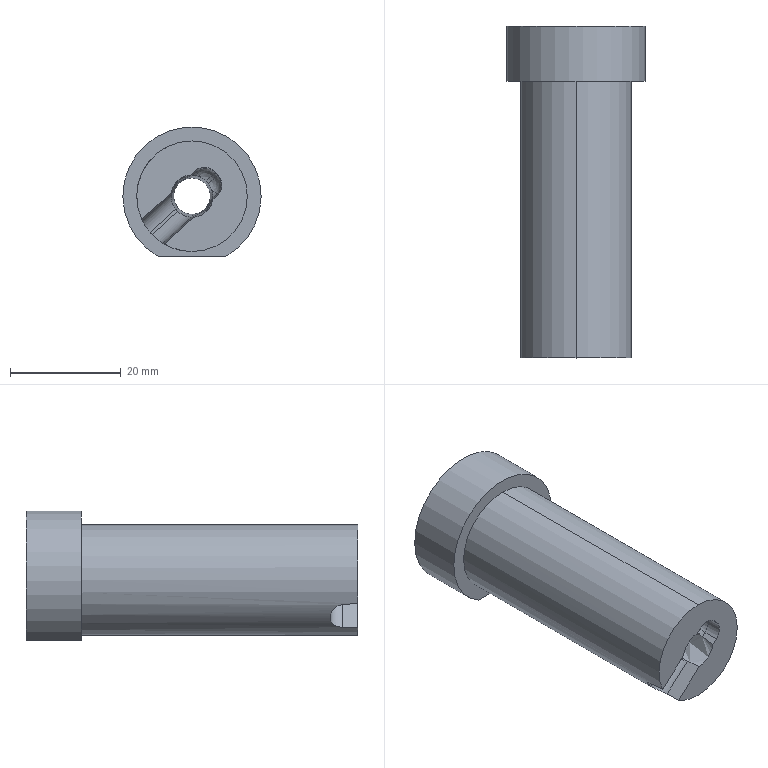Part | STEP file | 1 solid | 25 faces | box 25 x 60 x 23.412 mm | volume 17876 mm3 | cylinder 11 | plane 10 | cone 2 | sphere 2 | commonest cylinder face diameters 5 x8 20 x2 25 x1